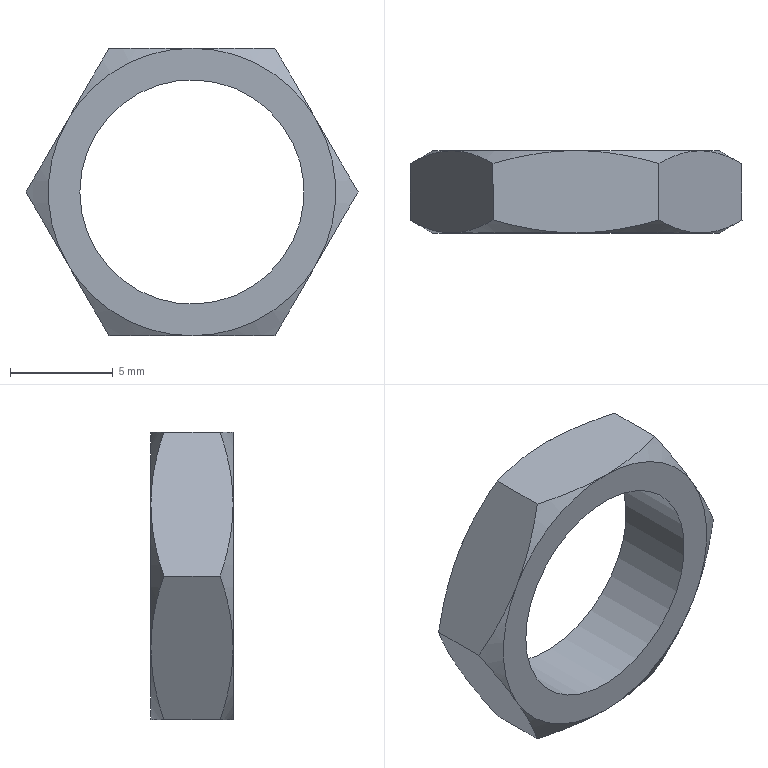Part | NX | features NAT_5003_027_C-AC1210S-N_1 2 | 1 solid | 21 faces | box 16.166 x 4 x 14 mm | volume 298.505 mm3 | cone 12 | plane 8 | cylinder 1 | commonest cylinder face diameters 10.917 x1
STEP:
#1=CARTESIAN_POINT('',(116.067,27.6,-122.));
#2=VERTEX_POINT('',#1);
#3=CARTESIAN_POINT('',(121.525,27.6,-122.));
#4=DIRECTION('',(0.,1.,0.));
#5=DIRECTION('',(-1.,0.,0.));
#6=AXIS2_PLACEMENT_3D('',#3,#4,#5);
#7=CIRCLE('',#6,5.458);
#8=EDGE_CURVE('',#2,#2,#7,.T.);
#9=ORIENTED_EDGE('',*,*,#8,.F.);
#10=EDGE_LOOP('',(#9));
#11=FACE_BOUND('',#10,.T.);
#12=CARTESIAN_POINT('',(116.067,31.6,-122.));
#13=VERTEX_POINT('',#12);
#14=CARTESIAN_POINT('',(121.525,31.6,-122.));
#15=DIRECTION('',(0.,1.,0.));
#16=DIRECTION('',(-1.,0.,0.));
#17=AXIS2_PLACEMENT_3D('',#14,#15,#16);
#18=CIRCLE('',#17,5.458);
#19=EDGE_CURVE('',#13,#13,#18,.F.);
#20=ORIENTED_EDGE('',*,*,#19,.F.);
#21=EDGE_LOOP('',(#20));
#22=FACE_BOUND('',#21,.T.);
#23=CARTESIAN_POINT('',(121.525,31.6,-122.));
#24=DIRECTION('',(0.,1.,0.));
#25=DIRECTION('',(-1.,0.,0.));
#26=AXIS2_PLACEMENT_3D('',#23,#24,#25);
#27=CYLINDRICAL_SURFACE('',#26,5.458);
#28=ADVANCED_FACE('',(#11,#22),#27,.F.);
#29=CARTESIAN_POINT('',(115.463,27.6,-125.5));
#30=VERTEX_POINT('',#29);
#31=CARTESIAN_POINT('',(115.463,27.6,-118.5));
#32=VERTEX_POINT('',#31);
#33=CARTESIAN_POINT('',(121.525,27.6,-122.));
#34=DIRECTION('',(0.,1.,0.));
#35=DIRECTION('',(-1.,0.,0.));
#36=AXIS2_PLACEMENT_3D('',#33,#34,#35);
#37=CIRCLE('',#36,7.);
#38=EDGE_CURVE('',#30,#32,#37,.T.);
#39=ORIENTED_EDGE('',*,*,#38,.F.);
#40=CARTESIAN_POINT('',(121.525,27.6,-129.));
#41=VERTEX_POINT('',#40);
#42=CARTESIAN_POINT('',(121.525,27.6,-122.));
#43=DIRECTION('',(0.,1.,0.));
#44=DIRECTION('',(-1.,0.,0.));
#45=AXIS2_PLACEMENT_3D('',#42,#43,#44);
#46=CIRCLE('',#45,7.);
#47=EDGE_CURVE('',#41,#30,#46,.T.);
#48=ORIENTED_EDGE('',*,*,#47,.F.);
#49=CARTESIAN_POINT('',(127.587,27.6,-125.5));
#50=VERTEX_POINT('',#49);
#51=CARTESIAN_POINT('',(121.525,27.6,-122.));
#52=DIRECTION('',(0.,1.,0.));
#53=DIRECTION('',(-1.,0.,0.));
#54=AXIS2_PLACEMENT_3D('',#51,#52,#53);
#55=CIRCLE('',#54,7.);
#56=EDGE_CURVE('',#50,#41,#55,.T.);
#57=ORIENTED_EDGE('',*,*,#56,.F.);
#58=CARTESIAN_POINT('',(127.587,27.6,-118.5));
#59=VERTEX_POINT('',#58);
#60=CARTESIAN_POINT('',(121.525,27.6,-122.));
#61=DIRECTION('',(0.,1.,0.));
#62=DIRECTION('',(-1.,0.,0.));
#63=AXIS2_PLACEMENT_3D('',#60,#61,#62);
#64=CIRCLE('',#63,7.);
#65=EDGE_CURVE('',#59,#50,#64,.T.);
#66=ORIENTED_EDGE('',*,*,#65,.F.);
#67=CARTESIAN_POINT('',(121.525,27.6,-115.));
#68=VERTEX_POINT('',#67);
#69=CARTESIAN_POINT('',(121.525,27.6,-122.));
#70=DIRECTION('',(0.,1.,0.));
#71=DIRECTION('',(-1.,0.,0.));
#72=AXIS2_PLACEMENT_3D('',#69,#70,#71);
#73=CIRCLE('',#72,7.);
#74=EDGE_CURVE('',#68,#59,#73,.T.);
#75=ORIENTED_EDGE('',*,*,#74,.F.);
#76=CARTESIAN_POINT('',(121.525,27.6,-122.));
#77=DIRECTION('',(0.,1.,0.));
#78=DIRECTION('',(-1.,0.,0.));
#79=AXIS2_PLACEMENT_3D('',#76,#77,#78);
#80=CIRCLE('',#79,7.);
#81=EDGE_CURVE('',#32,#68,#80,.T.);
#82=ORIENTED_EDGE('',*,*,#81,.F.);
#83=EDGE_LOOP('',(#39,#48,#57,#66,#75,#82));
#84=FACE_BOUND('',#83,.T.);
#85=ORIENTED_EDGE('',*,*,#8,.T.);
#86=EDGE_LOOP('',(#85));
#87=FACE_BOUND('',#86,.T.);
#88=CARTESIAN_POINT('',(121.525,27.6,-122.));
#89=DIRECTION('',(0.,1.,0.));
#90=DIRECTION('',(-1.,0.,0.));
#91=AXIS2_PLACEMENT_3D('',#88,#89,#90);
#92=PLANE('',#91);
#93=ADVANCED_FACE('',(#84,#87),#92,.F.);
#94=CARTESIAN_POINT('',(127.587,31.6,-125.5));
#95=VERTEX_POINT('',#94);
#96=CARTESIAN_POINT('',(121.525,31.6,-129.));
#97=VERTEX_POINT('',#96);
#98=CARTESIAN_POINT('',(121.525,31.6,-122.));
#99=DIRECTION('',(0.,-1.,0.));
#100=DIRECTION('',(0.,0.,-1.));
#101=AXIS2_PLACEMENT_3D('',#98,#99,#100);
#102=CIRCLE('',#101,7.);
#103=EDGE_CURVE('',#95,#97,#102,.F.);
#104=ORIENTED_EDGE('',*,*,#103,.T.);
#105=CARTESIAN_POINT('',(115.463,31.6,-125.5));
#106=VERTEX_POINT('',#105);
#107=CARTESIAN_POINT('',(121.525,31.6,-122.));
#108=DIRECTION('',(0.,-1.,0.));
#109=DIRECTION('',(0.,0.,-1.));
#110=AXIS2_PLACEMENT_3D('',#107,#108,#109);
#111=CIRCLE('',#110,7.);
#112=EDGE_CURVE('',#97,#106,#111,.F.);
#113=ORIENTED_EDGE('',*,*,#112,.T.);
#114=CARTESIAN_POINT('',(115.463,31.6,-118.5));
#115=VERTEX_POINT('',#114);
#116=CARTESIAN_POINT('',(121.525,31.6,-122.));
#117=DIRECTION('',(0.,-1.,0.));
#118=DIRECTION('',(1.,0.,0.));
#119=AXIS2_PLACEMENT_3D('',#116,#117,#118);
#120=CIRCLE('',#119,7.);
#121=EDGE_CURVE('',#106,#115,#120,.F.);
#122=ORIENTED_EDGE('',*,*,#121,.T.);
#123=CARTESIAN_POINT('',(121.525,31.6,-115.));
#124=VERTEX_POINT('',#123);
#125=CARTESIAN_POINT('',(121.525,31.6,-122.));
#126=DIRECTION('',(0.,-1.,0.));
#127=DIRECTION('',(0.,0.,-1.));
#128=AXIS2_PLACEMENT_3D('',#125,#126,#127);
#129=CIRCLE('',#128,7.);
#130=EDGE_CURVE('',#115,#124,#129,.F.);
#131=ORIENTED_EDGE('',*,*,#130,.T.);
#132=CARTESIAN_POINT('',(127.587,31.6,-118.5));
#133=VERTEX_POINT('',#132);
#134=CARTESIAN_POINT('',(121.525,31.6,-122.));
#135=DIRECTION('',(0.,-1.,0.));
#136=DIRECTION('',(1.,0.,0.));
#137=AXIS2_PLACEMENT_3D('',#134,#135,#136);
#138=CIRCLE('',#137,7.);
#139=EDGE_CURVE('',#124,#133,#138,.F.);
#140=ORIENTED_EDGE('',*,*,#139,.T.);
#141=CARTESIAN_POINT('',(121.525,31.6,-122.));
#142=DIRECTION('',(0.,-1.,0.));
#143=DIRECTION('',(1.,0.,0.));
#144=AXIS2_PLACEMENT_3D('',#141,#142,#143);
#145=CIRCLE('',#144,7.);
#146=EDGE_CURVE('',#133,#95,#145,.F.);
#147=ORIENTED_EDGE('',*,*,#146,.T.);
#148=EDGE_LOOP('',(#104,#113,#122,#131,#140,#147));
#149=FACE_BOUND('',#148,.T.);
#150=ORIENTED_EDGE('',*,*,#19,.T.);
#151=EDGE_LOOP('',(#150));
#152=FACE_BOUND('',#151,.T.);
#153=CARTESIAN_POINT('',(121.525,31.6,-122.));
#154=DIRECTION('',(0.,1.,0.));
#155=DIRECTION('',(-1.,0.,0.));
#156=AXIS2_PLACEMENT_3D('',#153,#154,#155);
#157=PLANE('',#156);
#158=ADVANCED_FACE('',(#149,#152),#157,.T.);
#159=CARTESIAN_POINT('',(117.484,28.225,-115.));
#160=VERTEX_POINT('',#159);
#161=CARTESIAN_POINT('',(117.484,28.225,-115.));
#162=CARTESIAN_POINT('',(116.823,27.844,-116.144));
#163=CARTESIAN_POINT('',(116.153,27.6,-117.305));
#164=CARTESIAN_POINT('',(115.463,27.6,-118.5));
#165=B_SPLINE_CURVE_WITH_KNOTS('',3,(#161,#162,#163,#164),.UNSPECIFIED.,.F.,.F.,(4,4),(0.,0.00409),.UNSPECIFIED.);
#166=EDGE_CURVE('',#160,#32,#165,.T.);
#167=ORIENTED_EDGE('',*,*,#166,.T.);
#168=ORIENTED_EDGE('',*,*,#81,.T.);
#169=CARTESIAN_POINT('',(121.525,27.6,-115.));
#170=CARTESIAN_POINT('',(120.146,27.6,-115.));
#171=CARTESIAN_POINT('',(118.804,27.844,-115.));
#172=CARTESIAN_POINT('',(117.484,28.225,-115.));
#173=B_SPLINE_CURVE_WITH_KNOTS('',3,(#169,#170,#171,#172),.UNSPECIFIED.,.F.,.F.,(4,4),(0.,0.00409),.UNSPECIFIED.);
#174=EDGE_CURVE('',#68,#160,#173,.T.);
#175=ORIENTED_EDGE('',*,*,#174,.T.);
#176=EDGE_LOOP('',(#167,#168,#175));
#177=FACE_BOUND('',#176,.T.);
#178=CARTESIAN_POINT('',(121.525,28.229,-122.));
#179=DIRECTION('',(0.,1.,0.));
#180=DIRECTION('',(-1.,0.,0.));
#181=AXIS2_PLACEMENT_3D('',#178,#179,#180);
#182=CONICAL_SURFACE('',#181,8.089,1.047);
#183=ADVANCED_FACE('',(#177),#182,.T.);
#184=ORIENTED_EDGE('',*,*,#38,.T.);
#185=CARTESIAN_POINT('',(113.442,28.225,-122.));
#186=VERTEX_POINT('',#185);
#187=CARTESIAN_POINT('',(115.463,27.6,-118.5));
#188=CARTESIAN_POINT('',(114.773,27.6,-119.695));
#189=CARTESIAN_POINT('',(114.102,27.844,-120.856));
#190=CARTESIAN_POINT('',(113.442,28.225,-122.));
#191=B_SPLINE_CURVE_WITH_KNOTS('',3,(#187,#188,#189,#190),.UNSPECIFIED.,.F.,.F.,(4,4),(0.,0.00409),.UNSPECIFIED.);
#192=EDGE_CURVE('',#32,#186,#191,.T.);
#193=ORIENTED_EDGE('',*,*,#192,.T.);
#194=CARTESIAN_POINT('',(113.442,28.225,-122.));
#195=CARTESIAN_POINT('',(114.102,27.844,-123.144));
#196=CARTESIAN_POINT('',(114.773,27.6,-124.305));
#197=CARTESIAN_POINT('',(115.463,27.6,-125.5));
#198=B_SPLINE_CURVE_WITH_KNOTS('',3,(#194,#195,#196,#197),.UNSPECIFIED.,.F.,.F.,(4,4),(0.,0.00409),.UNSPECIFIED.);
#199=EDGE_CURVE('',#186,#30,#198,.T.);
#200=ORIENTED_EDGE('',*,*,#199,.T.);
#201=EDGE_LOOP('',(#184,#193,#200));
#202=FACE_BOUND('',#201,.T.);
#203=CARTESIAN_POINT('',(121.525,28.229,-122.));
#204=DIRECTION('',(0.,1.,0.));
#205=DIRECTION('',(-1.,0.,0.));
#206=AXIS2_PLACEMENT_3D('',#203,#204,#205);
#207=CONICAL_SURFACE('',#206,8.089,1.047);
#208=ADVANCED_FACE('',(#202),#207,.T.);
#209=CARTESIAN_POINT('',(117.484,28.225,-129.));
#210=VERTEX_POINT('',#209);
#211=CARTESIAN_POINT('',(117.484,28.225,-129.));
#212=CARTESIAN_POINT('',(118.804,27.844,-129.));
#213=CARTESIAN_POINT('',(120.146,27.6,-129.));
#214=CARTESIAN_POINT('',(121.525,27.6,-129.));
#215=B_SPLINE_CURVE_WITH_KNOTS('',3,(#211,#212,#213,#214),.UNSPECIFIED.,.F.,.F.,(4,4),(0.,0.00409),.UNSPECIFIED.);
#216=EDGE_CURVE('',#210,#41,#215,.T.);
#217=ORIENTED_EDGE('',*,*,#216,.T.);
#218=ORIENTED_EDGE('',*,*,#47,.T.);
#219=CARTESIAN_POINT('',(115.463,27.6,-125.5));
#220=CARTESIAN_POINT('',(116.153,27.6,-126.695));
#221=CARTESIAN_POINT('',(116.823,27.844,-127.856));
#222=CARTESIAN_POINT('',(117.484,28.225,-129.));
#223=B_SPLINE_CURVE_WITH_KNOTS('',3,(#219,#220,#221,#222),.UNSPECIFIED.,.F.,.F.,(4,4),(0.,0.00409),.UNSPECIFIED.);
#224=EDGE_CURVE('',#30,#210,#223,.T.);
#225=ORIENTED_EDGE('',*,*,#224,.T.);
#226=EDGE_LOOP('',(#217,#218,#225));
#227=FACE_BOUND('',#226,.T.);
#228=CARTESIAN_POINT('',(121.525,28.229,-122.));
#229=DIRECTION('',(0.,1.,0.));
#230=DIRECTION('',(-1.,0.,0.));
#231=AXIS2_PLACEMENT_3D('',#228,#229,#230);
#232=CONICAL_SURFACE('',#231,8.089,1.047);
#233=ADVANCED_FACE('',(#227),#232,.T.);
#234=ORIENTED_EDGE('',*,*,#56,.T.);
#235=CARTESIAN_POINT('',(125.566,28.225,-129.));
#236=VERTEX_POINT('',#235);
#237=CARTESIAN_POINT('',(121.525,27.6,-129.));
#238=CARTESIAN_POINT('',(122.904,27.6,-129.));
#239=CARTESIAN_POINT('',(124.246,27.844,-129.));
#240=CARTESIAN_POINT('',(125.566,28.225,-129.));
#241=B_SPLINE_CURVE_WITH_KNOTS('',3,(#237,#238,#239,#240),.UNSPECIFIED.,.F.,.F.,(4,4),(0.,0.00409),.UNSPECIFIED.);
#242=EDGE_CURVE('',#41,#236,#241,.T.);
#243=ORIENTED_EDGE('',*,*,#242,.T.);
#244=CARTESIAN_POINT('',(125.566,28.225,-129.));
#245=CARTESIAN_POINT('',(126.227,27.844,-127.856));
#246=CARTESIAN_POINT('',(126.897,27.6,-126.695));
#247=CARTESIAN_POINT('',(127.587,27.6,-125.5));
#248=B_SPLINE_CURVE_WITH_KNOTS('',3,(#244,#245,#246,#247),.UNSPECIFIED.,.F.,.F.,(4,4),(0.,0.00409),.UNSPECIFIED.);
#249=EDGE_CURVE('',#236,#50,#248,.T.);
#250=ORIENTED_EDGE('',*,*,#249,.T.);
#251=EDGE_LOOP('',(#234,#243,#250));
#252=FACE_BOUND('',#251,.T.);
#253=CARTESIAN_POINT('',(121.525,28.229,-122.));
#254=DIRECTION('',(0.,1.,0.));
#255=DIRECTION('',(-1.,0.,0.));
#256=AXIS2_PLACEMENT_3D('',#253,#254,#255);
#257=CONICAL_SURFACE('',#256,8.089,1.047);
#258=ADVANCED_FACE('',(#252),#257,.T.);
#259=ORIENTED_EDGE('',*,*,#65,.T.);
#260=CARTESIAN_POINT('',(129.608,28.225,-122.));
#261=VERTEX_POINT('',#260);
#262=CARTESIAN_POINT('',(127.587,27.6,-125.5));
#263=CARTESIAN_POINT('',(128.277,27.6,-124.305));
#264=CARTESIAN_POINT('',(128.948,27.844,-123.144));
#265=CARTESIAN_POINT('',(129.608,28.225,-122.));
#266=B_SPLINE_CURVE_WITH_KNOTS('',3,(#262,#263,#264,#265),.UNSPECIFIED.,.F.,.F.,(4,4),(0.,0.00409),.UNSPECIFIED.);
#267=EDGE_CURVE('',#50,#261,#266,.T.);
#268=ORIENTED_EDGE('',*,*,#267,.T.);
#269=CARTESIAN_POINT('',(129.608,28.225,-122.));
#270=CARTESIAN_POINT('',(128.948,27.844,-120.856));
#271=CARTESIAN_POINT('',(128.277,27.6,-119.695));
#272=CARTESIAN_POINT('',(127.587,27.6,-118.5));
#273=B_SPLINE_CURVE_WITH_KNOTS('',3,(#269,#270,#271,#272),.UNSPECIFIED.,.F.,.F.,(4,4),(0.,0.00409),.UNSPECIFIED.);
#274=EDGE_CURVE('',#261,#59,#273,.T.);
#275=ORIENTED_EDGE('',*,*,#274,.T.);
#276=EDGE_LOOP('',(#259,#268,#275));
#277=FACE_BOUND('',#276,.T.);
#278=CARTESIAN_POINT('',(121.525,28.229,-122.));
#279=DIRECTION('',(0.,1.,0.));
#280=DIRECTION('',(-1.,0.,0.));
#281=AXIS2_PLACEMENT_3D('',#278,#279,#280);
#282=CONICAL_SURFACE('',#281,8.089,1.047);
#283=ADVANCED_FACE('',(#277),#282,.T.);
#284=ORIENTED_EDGE('',*,*,#74,.T.);
#285=CARTESIAN_POINT('',(125.566,28.225,-115.));
#286=VERTEX_POINT('',#285);
#287=CARTESIAN_POINT('',(127.587,27.6,-118.5));
#288=CARTESIAN_POINT('',(126.897,27.6,-117.305));
#289=CARTESIAN_POINT('',(126.227,27.844,-116.144));
#290=CARTESIAN_POINT('',(125.566,28.225,-115.));
#291=B_SPLINE_CURVE_WITH_KNOTS('',3,(#287,#288,#289,#290),.UNSPECIFIED.,.F.,.F.,(4,4),(0.,0.00409),.UNSPECIFIED.);
#292=EDGE_CURVE('',#59,#286,#291,.T.);
#293=ORIENTED_EDGE('',*,*,#292,.T.);
#294=CARTESIAN_POINT('',(125.566,28.225,-115.));
#295=CARTESIAN_POINT('',(124.246,27.844,-115.));
#296=CARTESIAN_POINT('',(122.904,27.6,-115.));
#297=CARTESIAN_POINT('',(121.525,27.6,-115.));
#298=B_SPLINE_CURVE_WITH_KNOTS('',3,(#294,#295,#296,#297),.UNSPECIFIED.,.F.,.F.,(4,4),(0.,0.00409),.UNSPECIFIED.);
#299=EDGE_CURVE('',#286,#68,#298,.T.);
#300=ORIENTED_EDGE('',*,*,#299,.T.);
#301=EDGE_LOOP('',(#284,#293,#300));
#302=FACE_BOUND('',#301,.T.);
#303=CARTESIAN_POINT('',(121.525,28.229,-122.));
#304=DIRECTION('',(0.,1.,0.));
#305=DIRECTION('',(-1.,0.,0.));
#306=AXIS2_PLACEMENT_3D('',#303,#304,#305);
#307=CONICAL_SURFACE('',#306,8.089,1.047);
#308=ADVANCED_FACE('',(#302),#307,.T.);
#309=ORIENTED_EDGE('',*,*,#112,.F.);
#310=CARTESIAN_POINT('',(117.484,30.975,-129.));
#311=VERTEX_POINT('',#310);
#312=CARTESIAN_POINT('',(121.525,31.6,-129.));
#313=CARTESIAN_POINT('',(120.146,31.6,-129.));
#314=CARTESIAN_POINT('',(118.804,31.356,-129.));
#315=CARTESIAN_POINT('',(117.484,30.975,-129.));
#316=B_SPLINE_CURVE_WITH_KNOTS('',3,(#312,#313,#314,#315),.UNSPECIFIED.,.F.,.F.,(4,4),(0.,0.00409),.UNSPECIFIED.);
#317=EDGE_CURVE('',#97,#311,#316,.T.);
#318=ORIENTED_EDGE('',*,*,#317,.T.);
#319=CARTESIAN_POINT('',(117.484,30.975,-129.));
#320=CARTESIAN_POINT('',(116.823,31.356,-127.856));
#321=CARTESIAN_POINT('',(116.153,31.6,-126.695));
#322=CARTESIAN_POINT('',(115.463,31.6,-125.5));
#323=B_SPLINE_CURVE_WITH_KNOTS('',3,(#319,#320,#321,#322),.UNSPECIFIED.,.F.,.F.,(4,4),(0.,0.00409),.UNSPECIFIED.);
#324=EDGE_CURVE('',#311,#106,#323,.T.);
#325=ORIENTED_EDGE('',*,*,#324,.T.);
#326=EDGE_LOOP('',(#309,#318,#325));
#327=FACE_BOUND('',#326,.T.);
#328=CARTESIAN_POINT('',(121.525,30.971,-122.));
#329=DIRECTION('',(0.,-1.,0.));
#330=DIRECTION('',(0.,0.,-1.));
#331=AXIS2_PLACEMENT_3D('',#328,#329,#330);
#332=CONICAL_SURFACE('',#331,8.089,1.047);
#333=ADVANCED_FACE('',(#327),#332,.T.);
#334=CARTESIAN_POINT('',(125.566,30.975,-129.));
#335=VERTEX_POINT('',#334);
#336=CARTESIAN_POINT('',(125.566,30.975,-129.));
#337=CARTESIAN_POINT('',(124.246,31.356,-129.));
#338=CARTESIAN_POINT('',(122.904,31.6,-129.));
#339=CARTESIAN_POINT('',(121.525,31.6,-129.));
#340=B_SPLINE_CURVE_WITH_KNOTS('',3,(#336,#337,#338,#339),.UNSPECIFIED.,.F.,.F.,(4,4),(0.,0.00409),.UNSPECIFIED.);
#341=EDGE_CURVE('',#335,#97,#340,.T.);
#342=ORIENTED_EDGE('',*,*,#341,.T.);
#343=ORIENTED_EDGE('',*,*,#103,.F.);
#344=CARTESIAN_POINT('',(127.587,31.6,-125.5));
#345=CARTESIAN_POINT('',(126.897,31.6,-126.695));
#346=CARTESIAN_POINT('',(126.227,31.356,-127.856));
#347=CARTESIAN_POINT('',(125.566,30.975,-129.));
#348=B_SPLINE_CURVE_WITH_KNOTS('',3,(#344,#345,#346,#347),.UNSPECIFIED.,.F.,.F.,(4,4),(0.,0.00409),.UNSPECIFIED.);
#349=EDGE_CURVE('',#95,#335,#348,.T.);
#350=ORIENTED_EDGE('',*,*,#349,.T.);
#351=EDGE_LOOP('',(#342,#343,#350));
#352=FACE_BOUND('',#351,.T.);
#353=CARTESIAN_POINT('',(121.525,30.971,-122.));
#354=DIRECTION('',(0.,-1.,0.));
#355=DIRECTION('',(0.,0.,-1.));
#356=AXIS2_PLACEMENT_3D('',#353,#354,#355);
#357=CONICAL_SURFACE('',#356,8.089,1.047);
#358=ADVANCED_FACE('',(#352),#357,.T.);
#359=ORIENTED_EDGE('',*,*,#146,.F.);
#360=CARTESIAN_POINT('',(129.608,30.975,-122.));
#361=VERTEX_POINT('',#360);
#362=CARTESIAN_POINT('',(127.587,31.6,-118.5));
#363=CARTESIAN_POINT('',(128.277,31.6,-119.695));
#364=CARTESIAN_POINT('',(128.948,31.356,-120.856));
#365=CARTESIAN_POINT('',(129.608,30.975,-122.));
#366=B_SPLINE_CURVE_WITH_KNOTS('',3,(#362,#363,#364,#365),.UNSPECIFIED.,.F.,.F.,(4,4),(0.,0.00409),.UNSPECIFIED.);
#367=EDGE_CURVE('',#133,#361,#366,.T.);
#368=ORIENTED_EDGE('',*,*,#367,.T.);
#369=CARTESIAN_POINT('',(129.608,30.975,-122.));
#370=CARTESIAN_POINT('',(128.948,31.356,-123.144));
#371=CARTESIAN_POINT('',(128.277,31.6,-124.305));
#372=CARTESIAN_POINT('',(127.587,31.6,-125.5));
#373=B_SPLINE_CURVE_WITH_KNOTS('',3,(#369,#370,#371,#372),.UNSPECIFIED.,.F.,.F.,(4,4),(0.,0.00409),.UNSPECIFIED.);
#374=EDGE_CURVE('',#361,#95,#373,.T.);
#375=ORIENTED_EDGE('',*,*,#374,.T.);
#376=EDGE_LOOP('',(#359,#368,#375));
#377=FACE_BOUND('',#376,.T.);
#378=CARTESIAN_POINT('',(121.525,30.971,-122.));
#379=DIRECTION('',(0.,-1.,0.));
#380=DIRECTION('',(1.,0.,0.));
#381=AXIS2_PLACEMENT_3D('',#378,#379,#380);
#382=CONICAL_SURFACE('',#381,8.089,1.047);
#383=ADVANCED_FACE('',(#377),#382,.T.);
#384=CARTESIAN_POINT('',(125.566,30.975,-115.));
#385=VERTEX_POINT('',#384);
#386=CARTESIAN_POINT('',(125.566,30.975,-115.));
#387=CARTESIAN_POINT('',(126.227,31.356,-116.144));
#388=CARTESIAN_POINT('',(126.897,31.6,-117.305));
#389=CARTESIAN_POINT('',(127.587,31.6,-118.5));
#390=B_SPLINE_CURVE_WITH_KNOTS('',3,(#386,#387,#388,#389),.UNSPECIFIED.,.F.,.F.,(4,4),(0.,0.00409),.UNSPECIFIED.);
#391=EDGE_CURVE('',#385,#133,#390,.T.);
#392=ORIENTED_EDGE('',*,*,#391,.T.);
#393=ORIENTED_EDGE('',*,*,#139,.F.);
#394=CARTESIAN_POINT('',(121.525,31.6,-115.));
#395=CARTESIAN_POINT('',(122.904,31.6,-115.));
#396=CARTESIAN_POINT('',(124.246,31.356,-115.));
#397=CARTESIAN_POINT('',(125.566,30.975,-115.));
#398=B_SPLINE_CURVE_WITH_KNOTS('',3,(#394,#395,#396,#397),.UNSPECIFIED.,.F.,.F.,(4,4),(0.,0.00409),.UNSPECIFIED.);
#399=EDGE_CURVE('',#124,#385,#398,.T.);
#400=ORIENTED_EDGE('',*,*,#399,.T.);
#401=EDGE_LOOP('',(#392,#393,#400));
#402=FACE_BOUND('',#401,.T.);
#403=CARTESIAN_POINT('',(121.525,30.971,-122.));
#404=DIRECTION('',(0.,-1.,0.));
#405=DIRECTION('',(1.,0.,0.));
#406=AXIS2_PLACEMENT_3D('',#403,#404,#405);
#407=CONICAL_SURFACE('',#406,8.089,1.047);
#408=ADVANCED_FACE('',(#402),#407,.T.);
#409=CARTESIAN_POINT('',(117.484,30.975,-115.));
#410=VERTEX_POINT('',#409);
#411=CARTESIAN_POINT('',(117.484,30.975,-115.));
#412=CARTESIAN_POINT('',(118.804,31.356,-115.));
#413=CARTESIAN_POINT('',(120.146,31.6,-115.));
#414=CARTESIAN_POINT('',(121.525,31.6,-115.));
#415=B_SPLINE_CURVE_WITH_KNOTS('',3,(#411,#412,#413,#414),.UNSPECIFIED.,.F.,.F.,(4,4),(0.,0.00409),.UNSPECIFIED.);
#416=EDGE_CURVE('',#410,#124,#415,.T.);
#417=ORIENTED_EDGE('',*,*,#416,.T.);
#418=ORIENTED_EDGE('',*,*,#130,.F.);
#419=CARTESIAN_POINT('',(115.463,31.6,-118.5));
#420=CARTESIAN_POINT('',(116.153,31.6,-117.305));
#421=CARTESIAN_POINT('',(116.823,31.356,-116.144));
#422=CARTESIAN_POINT('',(117.484,30.975,-115.));
#423=B_SPLINE_CURVE_WITH_KNOTS('',3,(#419,#420,#421,#422),.UNSPECIFIED.,.F.,.F.,(4,4),(0.,0.00409),.UNSPECIFIED.);
#424=EDGE_CURVE('',#115,#410,#423,.T.);
#425=ORIENTED_EDGE('',*,*,#424,.T.);
#426=EDGE_LOOP('',(#417,#418,#425));
#427=FACE_BOUND('',#426,.T.);
#428=CARTESIAN_POINT('',(121.525,30.971,-122.));
#429=DIRECTION('',(0.,-1.,0.));
#430=DIRECTION('',(0.,0.,-1.));
#431=AXIS2_PLACEMENT_3D('',#428,#429,#430);
#432=CONICAL_SURFACE('',#431,8.089,1.047);
#433=ADVANCED_FACE('',(#427),#432,.T.);
#434=CARTESIAN_POINT('',(113.442,30.975,-122.));
#435=VERTEX_POINT('',#434);
#436=CARTESIAN_POINT('',(113.442,30.975,-122.));
#437=CARTESIAN_POINT('',(114.102,31.356,-120.856));
#438=CARTESIAN_POINT('',(114.773,31.6,-119.695));
#439=CARTESIAN_POINT('',(115.463,31.6,-118.5));
#440=B_SPLINE_CURVE_WITH_KNOTS('',3,(#436,#437,#438,#439),.UNSPECIFIED.,.F.,.F.,(4,4),(0.,0.00409),.UNSPECIFIED.);
#441=EDGE_CURVE('',#435,#115,#440,.T.);
#442=ORIENTED_EDGE('',*,*,#441,.T.);
#443=ORIENTED_EDGE('',*,*,#121,.F.);
#444=CARTESIAN_POINT('',(115.463,31.6,-125.5));
#445=CARTESIAN_POINT('',(114.773,31.6,-124.305));
#446=CARTESIAN_POINT('',(114.102,31.356,-123.144));
#447=CARTESIAN_POINT('',(113.442,30.975,-122.));
#448=B_SPLINE_CURVE_WITH_KNOTS('',3,(#444,#445,#446,#447),.UNSPECIFIED.,.F.,.F.,(4,4),(0.,0.00409),.UNSPECIFIED.);
#449=EDGE_CURVE('',#106,#435,#448,.T.);
#450=ORIENTED_EDGE('',*,*,#449,.T.);
#451=EDGE_LOOP('',(#442,#443,#450));
#452=FACE_BOUND('',#451,.T.);
#453=CARTESIAN_POINT('',(121.525,30.971,-122.));
#454=DIRECTION('',(0.,-1.,0.));
#455=DIRECTION('',(1.,0.,0.));
#456=AXIS2_PLACEMENT_3D('',#453,#454,#455);
#457=CONICAL_SURFACE('',#456,8.089,1.047);
#458=ADVANCED_FACE('',(#452),#457,.T.);
#459=CARTESIAN_POINT('',(113.442,31.6,-122.));
#460=DIRECTION('',(0.,1.,0.));
#461=VECTOR('',#460,1000.);
#462=LINE('',#459,#461);
#463=EDGE_CURVE('',#186,#435,#462,.T.);
#464=ORIENTED_EDGE('',*,*,#463,.F.);
#465=ORIENTED_EDGE('',*,*,#192,.F.);
#466=ORIENTED_EDGE('',*,*,#166,.F.);
#467=CARTESIAN_POINT('',(117.484,31.6,-115.));
#468=DIRECTION('',(0.,1.,0.));
#469=VECTOR('',#468,1000.);
#470=LINE('',#467,#469);
#471=EDGE_CURVE('',#410,#160,#470,.F.);
#472=ORIENTED_EDGE('',*,*,#471,.F.);
#473=ORIENTED_EDGE('',*,*,#424,.F.);
#474=ORIENTED_EDGE('',*,*,#441,.F.);
#475=EDGE_LOOP('',(#464,#465,#466,#472,#473,#474));
#476=FACE_BOUND('',#475,.T.);
#477=CARTESIAN_POINT('',(113.442,31.6,-122.));
#478=DIRECTION('',(0.866,0.,-0.5));
#479=DIRECTION('',(-0.5,0.,-0.866));
#480=AXIS2_PLACEMENT_3D('',#477,#478,#479);
#481=PLANE('',#480);
#482=ADVANCED_FACE('',(#476),#481,.F.);
#483=ORIENTED_EDGE('',*,*,#471,.T.);
#484=ORIENTED_EDGE('',*,*,#174,.F.);
#485=ORIENTED_EDGE('',*,*,#299,.F.);
#486=CARTESIAN_POINT('',(125.566,31.6,-115.));
#487=DIRECTION('',(0.,1.,0.));
#488=VECTOR('',#487,1000.);
#489=LINE('',#486,#488);
#490=EDGE_CURVE('',#385,#286,#489,.F.);
#491=ORIENTED_EDGE('',*,*,#490,.F.);
#492=ORIENTED_EDGE('',*,*,#399,.F.);
#493=ORIENTED_EDGE('',*,*,#416,.F.);
#494=EDGE_LOOP('',(#483,#484,#485,#491,#492,#493));
#495=FACE_BOUND('',#494,.T.);
#496=CARTESIAN_POINT('',(117.484,31.6,-115.));
#497=DIRECTION('',(0.,0.,-1.));
#498=DIRECTION('',(-1.,0.,0.));
#499=AXIS2_PLACEMENT_3D('',#496,#497,#498);
#500=PLANE('',#499);
#501=ADVANCED_FACE('',(#495),#500,.F.);
#502=CARTESIAN_POINT('',(117.484,31.6,-129.));
#503=DIRECTION('',(0.,1.,0.));
#504=VECTOR('',#503,1000.);
#505=LINE('',#502,#504);
#506=EDGE_CURVE('',#210,#311,#505,.T.);
#507=ORIENTED_EDGE('',*,*,#506,.F.);
#508=ORIENTED_EDGE('',*,*,#224,.F.);
#509=ORIENTED_EDGE('',*,*,#199,.F.);
#510=ORIENTED_EDGE('',*,*,#463,.T.);
#511=ORIENTED_EDGE('',*,*,#449,.F.);
#512=ORIENTED_EDGE('',*,*,#324,.F.);
#513=EDGE_LOOP('',(#507,#508,#509,#510,#511,#512));
#514=FACE_BOUND('',#513,.T.);
#515=CARTESIAN_POINT('',(117.484,31.6,-129.));
#516=DIRECTION('',(0.866,0.,0.5));
#517=DIRECTION('',(0.5,0.,-0.866));
#518=AXIS2_PLACEMENT_3D('',#515,#516,#517);
#519=PLANE('',#518);
#520=ADVANCED_FACE('',(#514),#519,.F.);
#521=CARTESIAN_POINT('',(125.566,31.6,-129.));
#522=DIRECTION('',(0.,1.,0.));
#523=VECTOR('',#522,1000.);
#524=LINE('',#521,#523);
#525=EDGE_CURVE('',#236,#335,#524,.T.);
#526=ORIENTED_EDGE('',*,*,#525,.F.);
#527=ORIENTED_EDGE('',*,*,#242,.F.);
#528=ORIENTED_EDGE('',*,*,#216,.F.);
#529=ORIENTED_EDGE('',*,*,#506,.T.);
#530=ORIENTED_EDGE('',*,*,#317,.F.);
#531=ORIENTED_EDGE('',*,*,#341,.F.);
#532=EDGE_LOOP('',(#526,#527,#528,#529,#530,#531));
#533=FACE_BOUND('',#532,.T.);
#534=CARTESIAN_POINT('',(125.566,31.6,-129.));
#535=DIRECTION('',(0.,0.,1.));
#536=DIRECTION('',(1.,0.,0.));
#537=AXIS2_PLACEMENT_3D('',#534,#535,#536);
#538=PLANE('',#537);
#539=ADVANCED_FACE('',(#533),#538,.F.);
#540=CARTESIAN_POINT('',(129.608,31.6,-122.));
#541=DIRECTION('',(0.,1.,0.));
#542=VECTOR('',#541,1000.);
#543=LINE('',#540,#542);
#544=EDGE_CURVE('',#261,#361,#543,.T.);
#545=ORIENTED_EDGE('',*,*,#544,.F.);
#546=ORIENTED_EDGE('',*,*,#267,.F.);
#547=ORIENTED_EDGE('',*,*,#249,.F.);
#548=ORIENTED_EDGE('',*,*,#525,.T.);
#549=ORIENTED_EDGE('',*,*,#349,.F.);
#550=ORIENTED_EDGE('',*,*,#374,.F.);
#551=EDGE_LOOP('',(#545,#546,#547,#548,#549,#550));
#552=FACE_BOUND('',#551,.T.);
#553=CARTESIAN_POINT('',(129.608,31.6,-122.));
#554=DIRECTION('',(-0.866,0.,0.5));
#555=DIRECTION('',(0.5,0.,0.866));
#556=AXIS2_PLACEMENT_3D('',#553,#554,#555);
#557=PLANE('',#556);
#558=ADVANCED_FACE('',(#552),#557,.F.);
#559=ORIENTED_EDGE('',*,*,#490,.T.);
#560=ORIENTED_EDGE('',*,*,#292,.F.);
#561=ORIENTED_EDGE('',*,*,#274,.F.);
#562=ORIENTED_EDGE('',*,*,#544,.T.);
#563=ORIENTED_EDGE('',*,*,#367,.F.);
#564=ORIENTED_EDGE('',*,*,#391,.F.);
#565=EDGE_LOOP('',(#559,#560,#561,#562,#563,#564));
#566=FACE_BOUND('',#565,.T.);
#567=CARTESIAN_POINT('',(125.566,31.6,-115.));
#568=DIRECTION('',(-0.866,0.,-0.5));
#569=DIRECTION('',(-0.5,0.,0.866));
#570=AXIS2_PLACEMENT_3D('',#567,#568,#569);
#571=PLANE('',#570);
#572=ADVANCED_FACE('',(#566),#571,.F.);
#573=CLOSED_SHELL('',(#28,#93,#158,#183,#208,#233,#258,#283,#308,#333,#358,#383,#408,#433,#458,#482,#501,#520,#539,#558,#572));
#574=MANIFOLD_SOLID_BREP('',#573);
#575=(LENGTH_UNIT()NAMED_UNIT(*)SI_UNIT(.MILLI.,.METRE.));
#576=UNCERTAINTY_MEASURE_WITH_UNIT(LENGTH_MEASURE(0.0508),#575,'','');
#577=(NAMED_UNIT(*)PLANE_ANGLE_UNIT()SI_UNIT($,.RADIAN.));
#578=(NAMED_UNIT(*)SI_UNIT($,.STERADIAN.)SOLID_ANGLE_UNIT());
#579=(GEOMETRIC_REPRESENTATION_CONTEXT(3)GLOBAL_UNCERTAINTY_ASSIGNED_CONTEXT((#576))GLOBAL_UNIT_ASSIGNED_CONTEXT((#575,#577,#578))REPRESENTATION_CONTEXT('',''));
#580=ADVANCED_BREP_SHAPE_REPRESENTATION('',(#574),#579);